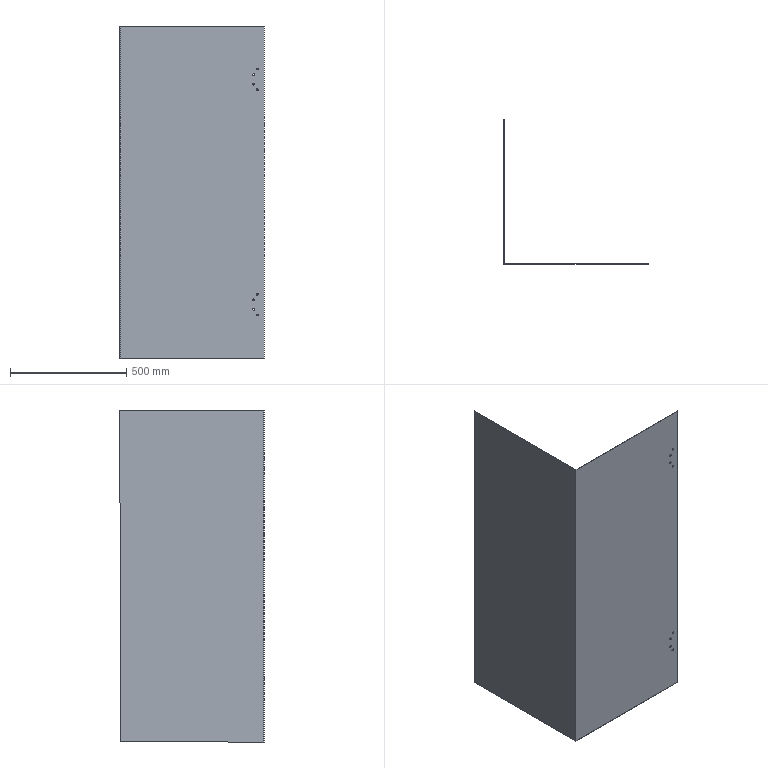Part | SolidWorks | features BaseBody 1 | 1 solid | 24 faces | box 620 x 620 x 1428 mm | volume 3533218 mm3 | cylinder 16 | plane 8 | commonest cylinder face diameters 8.5 x16
STEP:
#1=CARTESIAN_POINT('',(-23.395,-549.023,2695.25));
#2=VERTEX_POINT('',#1);
#3=CARTESIAN_POINT('',(-23.395,-549.023,2686.75));
#4=VERTEX_POINT('',#3);
#5=CARTESIAN_POINT('',(-23.395,-549.023,2691.));
#6=DIRECTION('',(0.,-1.,0.));
#7=DIRECTION('',(0.,0.,-1.));
#8=AXIS2_PLACEMENT_3D('',#5,#6,#7);
#9=CIRCLE('',#8,4.25);
#10=EDGE_CURVE('',#2,#4,#9,.T.);
#11=ORIENTED_EDGE('',*,*,#10,.F.);
#12=CARTESIAN_POINT('',(-23.395,-551.023,2695.25));
#13=VERTEX_POINT('',#12);
#14=CARTESIAN_POINT('',(-23.395,-551.023,2695.25));
#15=DIRECTION('',(0.,-1.,0.));
#16=VECTOR('',#15,1000.);
#17=LINE('',#14,#16);
#18=EDGE_CURVE('',#2,#13,#17,.T.);
#19=ORIENTED_EDGE('',*,*,#18,.T.);
#20=CARTESIAN_POINT('',(-23.395,-551.023,2686.75));
#21=VERTEX_POINT('',#20);
#22=CARTESIAN_POINT('',(-23.395,-551.023,2691.));
#23=DIRECTION('',(0.,-1.,0.));
#24=DIRECTION('',(0.,0.,-1.));
#25=AXIS2_PLACEMENT_3D('',#22,#23,#24);
#26=CIRCLE('',#25,4.25);
#27=EDGE_CURVE('',#13,#21,#26,.T.);
#28=ORIENTED_EDGE('',*,*,#27,.T.);
#29=CARTESIAN_POINT('',(-23.395,-551.023,2686.75));
#30=DIRECTION('',(0.,-1.,0.));
#31=VECTOR('',#30,1000.);
#32=LINE('',#29,#31);
#33=EDGE_CURVE('',#4,#21,#32,.T.);
#34=ORIENTED_EDGE('',*,*,#33,.F.);
#35=EDGE_LOOP('',(#11,#19,#28,#34));
#36=FACE_OUTER_BOUND('',#35,.T.);
#37=CARTESIAN_POINT('',(-23.395,-551.023,2691.));
#38=DIRECTION('',(0.,-1.,0.));
#39=DIRECTION('',(0.,0.,-1.));
#40=AXIS2_PLACEMENT_3D('',#37,#38,#39);
#41=CYLINDRICAL_SURFACE('',#40,4.25);
#42=ADVANCED_FACE('',(#36),#41,.F.);
#43=CARTESIAN_POINT('',(-38.395,-549.023,2670.25));
#44=VERTEX_POINT('',#43);
#45=CARTESIAN_POINT('',(-38.395,-549.023,2661.75));
#46=VERTEX_POINT('',#45);
#47=CARTESIAN_POINT('',(-38.395,-549.023,2666.));
#48=DIRECTION('',(0.,-1.,0.));
#49=DIRECTION('',(0.,0.,-1.));
#50=AXIS2_PLACEMENT_3D('',#47,#48,#49);
#51=CIRCLE('',#50,4.25);
#52=EDGE_CURVE('',#44,#46,#51,.T.);
#53=ORIENTED_EDGE('',*,*,#52,.F.);
#54=CARTESIAN_POINT('',(-38.395,-551.023,2670.25));
#55=VERTEX_POINT('',#54);
#56=CARTESIAN_POINT('',(-38.395,-551.023,2670.25));
#57=DIRECTION('',(0.,-1.,0.));
#58=VECTOR('',#57,1000.);
#59=LINE('',#56,#58);
#60=EDGE_CURVE('',#44,#55,#59,.T.);
#61=ORIENTED_EDGE('',*,*,#60,.T.);
#62=CARTESIAN_POINT('',(-38.395,-551.023,2661.75));
#63=VERTEX_POINT('',#62);
#64=CARTESIAN_POINT('',(-38.395,-551.023,2666.));
#65=DIRECTION('',(0.,-1.,0.));
#66=DIRECTION('',(0.,0.,-1.));
#67=AXIS2_PLACEMENT_3D('',#64,#65,#66);
#68=CIRCLE('',#67,4.25);
#69=EDGE_CURVE('',#55,#63,#68,.T.);
#70=ORIENTED_EDGE('',*,*,#69,.T.);
#71=CARTESIAN_POINT('',(-38.395,-551.023,2661.75));
#72=DIRECTION('',(0.,-1.,0.));
#73=VECTOR('',#72,1000.);
#74=LINE('',#71,#73);
#75=EDGE_CURVE('',#46,#63,#74,.T.);
#76=ORIENTED_EDGE('',*,*,#75,.F.);
#77=EDGE_LOOP('',(#53,#61,#70,#76));
#78=FACE_OUTER_BOUND('',#77,.T.);
#79=CARTESIAN_POINT('',(-38.395,-551.023,2666.));
#80=DIRECTION('',(0.,-1.,0.));
#81=DIRECTION('',(0.,0.,-1.));
#82=AXIS2_PLACEMENT_3D('',#79,#80,#81);
#83=CYLINDRICAL_SURFACE('',#82,4.25);
#84=ADVANCED_FACE('',(#78),#83,.F.);
#85=CARTESIAN_POINT('',(-38.395,-549.023,2630.25));
#86=VERTEX_POINT('',#85);
#87=CARTESIAN_POINT('',(-38.395,-549.023,2621.75));
#88=VERTEX_POINT('',#87);
#89=CARTESIAN_POINT('',(-38.395,-549.023,2626.));
#90=DIRECTION('',(0.,-1.,0.));
#91=DIRECTION('',(0.,0.,-1.));
#92=AXIS2_PLACEMENT_3D('',#89,#90,#91);
#93=CIRCLE('',#92,4.25);
#94=EDGE_CURVE('',#86,#88,#93,.T.);
#95=ORIENTED_EDGE('',*,*,#94,.F.);
#96=CARTESIAN_POINT('',(-38.395,-551.023,2630.25));
#97=VERTEX_POINT('',#96);
#98=CARTESIAN_POINT('',(-38.395,-551.023,2630.25));
#99=DIRECTION('',(0.,-1.,0.));
#100=VECTOR('',#99,1000.);
#101=LINE('',#98,#100);
#102=EDGE_CURVE('',#86,#97,#101,.T.);
#103=ORIENTED_EDGE('',*,*,#102,.T.);
#104=CARTESIAN_POINT('',(-38.395,-551.023,2621.75));
#105=VERTEX_POINT('',#104);
#106=CARTESIAN_POINT('',(-38.395,-551.023,2626.));
#107=DIRECTION('',(0.,-1.,0.));
#108=DIRECTION('',(0.,0.,-1.));
#109=AXIS2_PLACEMENT_3D('',#106,#107,#108);
#110=CIRCLE('',#109,4.25);
#111=EDGE_CURVE('',#97,#105,#110,.T.);
#112=ORIENTED_EDGE('',*,*,#111,.T.);
#113=CARTESIAN_POINT('',(-38.395,-551.023,2621.75));
#114=DIRECTION('',(0.,-1.,0.));
#115=VECTOR('',#114,1000.);
#116=LINE('',#113,#115);
#117=EDGE_CURVE('',#88,#105,#116,.T.);
#118=ORIENTED_EDGE('',*,*,#117,.F.);
#119=EDGE_LOOP('',(#95,#103,#112,#118));
#120=FACE_OUTER_BOUND('',#119,.T.);
#121=CARTESIAN_POINT('',(-38.395,-551.023,2626.));
#122=DIRECTION('',(0.,-1.,0.));
#123=DIRECTION('',(0.,0.,-1.));
#124=AXIS2_PLACEMENT_3D('',#121,#122,#123);
#125=CYLINDRICAL_SURFACE('',#124,4.25);
#126=ADVANCED_FACE('',(#120),#125,.F.);
#127=CARTESIAN_POINT('',(-23.395,-549.023,2605.25));
#128=VERTEX_POINT('',#127);
#129=CARTESIAN_POINT('',(-23.395,-549.023,2596.75));
#130=VERTEX_POINT('',#129);
#131=CARTESIAN_POINT('',(-23.395,-549.023,2601.));
#132=DIRECTION('',(0.,-1.,0.));
#133=DIRECTION('',(0.,0.,-1.));
#134=AXIS2_PLACEMENT_3D('',#131,#132,#133);
#135=CIRCLE('',#134,4.25);
#136=EDGE_CURVE('',#128,#130,#135,.T.);
#137=ORIENTED_EDGE('',*,*,#136,.F.);
#138=CARTESIAN_POINT('',(-23.395,-551.023,2605.25));
#139=VERTEX_POINT('',#138);
#140=CARTESIAN_POINT('',(-23.395,-551.023,2605.25));
#141=DIRECTION('',(0.,-1.,0.));
#142=VECTOR('',#141,1000.);
#143=LINE('',#140,#142);
#144=EDGE_CURVE('',#128,#139,#143,.T.);
#145=ORIENTED_EDGE('',*,*,#144,.T.);
#146=CARTESIAN_POINT('',(-23.395,-551.023,2596.75));
#147=VERTEX_POINT('',#146);
#148=CARTESIAN_POINT('',(-23.395,-551.023,2601.));
#149=DIRECTION('',(0.,-1.,0.));
#150=DIRECTION('',(0.,0.,-1.));
#151=AXIS2_PLACEMENT_3D('',#148,#149,#150);
#152=CIRCLE('',#151,4.25);
#153=EDGE_CURVE('',#139,#147,#152,.T.);
#154=ORIENTED_EDGE('',*,*,#153,.T.);
#155=CARTESIAN_POINT('',(-23.395,-551.023,2596.75));
#156=DIRECTION('',(0.,-1.,0.));
#157=VECTOR('',#156,1000.);
#158=LINE('',#155,#157);
#159=EDGE_CURVE('',#130,#147,#158,.T.);
#160=ORIENTED_EDGE('',*,*,#159,.F.);
#161=EDGE_LOOP('',(#137,#145,#154,#160));
#162=FACE_OUTER_BOUND('',#161,.T.);
#163=CARTESIAN_POINT('',(-23.395,-551.023,2601.));
#164=DIRECTION('',(0.,-1.,0.));
#165=DIRECTION('',(0.,0.,-1.));
#166=AXIS2_PLACEMENT_3D('',#163,#164,#165);
#167=CYLINDRICAL_SURFACE('',#166,4.25);
#168=ADVANCED_FACE('',(#162),#167,.F.);
#169=CARTESIAN_POINT('',(-23.395,-549.023,1727.25));
#170=VERTEX_POINT('',#169);
#171=CARTESIAN_POINT('',(-23.395,-549.023,1718.75));
#172=VERTEX_POINT('',#171);
#173=CARTESIAN_POINT('',(-23.395,-549.023,1723.));
#174=DIRECTION('',(0.,-1.,0.));
#175=DIRECTION('',(0.,0.,-1.));
#176=AXIS2_PLACEMENT_3D('',#173,#174,#175);
#177=CIRCLE('',#176,4.25);
#178=EDGE_CURVE('',#170,#172,#177,.T.);
#179=ORIENTED_EDGE('',*,*,#178,.F.);
#180=CARTESIAN_POINT('',(-23.395,-551.023,1727.25));
#181=VERTEX_POINT('',#180);
#182=CARTESIAN_POINT('',(-23.395,-551.023,1727.25));
#183=DIRECTION('',(0.,-1.,0.));
#184=VECTOR('',#183,1000.);
#185=LINE('',#182,#184);
#186=EDGE_CURVE('',#170,#181,#185,.T.);
#187=ORIENTED_EDGE('',*,*,#186,.T.);
#188=CARTESIAN_POINT('',(-23.395,-551.023,1718.75));
#189=VERTEX_POINT('',#188);
#190=CARTESIAN_POINT('',(-23.395,-551.023,1723.));
#191=DIRECTION('',(0.,-1.,0.));
#192=DIRECTION('',(0.,0.,-1.));
#193=AXIS2_PLACEMENT_3D('',#190,#191,#192);
#194=CIRCLE('',#193,4.25);
#195=EDGE_CURVE('',#181,#189,#194,.T.);
#196=ORIENTED_EDGE('',*,*,#195,.T.);
#197=CARTESIAN_POINT('',(-23.395,-551.023,1718.75));
#198=DIRECTION('',(0.,-1.,0.));
#199=VECTOR('',#198,1000.);
#200=LINE('',#197,#199);
#201=EDGE_CURVE('',#172,#189,#200,.T.);
#202=ORIENTED_EDGE('',*,*,#201,.F.);
#203=EDGE_LOOP('',(#179,#187,#196,#202));
#204=FACE_OUTER_BOUND('',#203,.T.);
#205=CARTESIAN_POINT('',(-23.395,-551.023,1723.));
#206=DIRECTION('',(0.,-1.,0.));
#207=DIRECTION('',(0.,0.,-1.));
#208=AXIS2_PLACEMENT_3D('',#205,#206,#207);
#209=CYLINDRICAL_SURFACE('',#208,4.25);
#210=ADVANCED_FACE('',(#204),#209,.F.);
#211=CARTESIAN_POINT('',(-38.395,-549.023,1702.25));
#212=VERTEX_POINT('',#211);
#213=CARTESIAN_POINT('',(-38.395,-549.023,1693.75));
#214=VERTEX_POINT('',#213);
#215=CARTESIAN_POINT('',(-38.395,-549.023,1698.));
#216=DIRECTION('',(0.,-1.,0.));
#217=DIRECTION('',(0.,0.,-1.));
#218=AXIS2_PLACEMENT_3D('',#215,#216,#217);
#219=CIRCLE('',#218,4.25);
#220=EDGE_CURVE('',#212,#214,#219,.T.);
#221=ORIENTED_EDGE('',*,*,#220,.F.);
#222=CARTESIAN_POINT('',(-38.395,-551.023,1702.25));
#223=VERTEX_POINT('',#222);
#224=CARTESIAN_POINT('',(-38.395,-551.023,1702.25));
#225=DIRECTION('',(0.,-1.,0.));
#226=VECTOR('',#225,1000.);
#227=LINE('',#224,#226);
#228=EDGE_CURVE('',#212,#223,#227,.T.);
#229=ORIENTED_EDGE('',*,*,#228,.T.);
#230=CARTESIAN_POINT('',(-38.395,-551.023,1693.75));
#231=VERTEX_POINT('',#230);
#232=CARTESIAN_POINT('',(-38.395,-551.023,1698.));
#233=DIRECTION('',(0.,-1.,0.));
#234=DIRECTION('',(0.,0.,-1.));
#235=AXIS2_PLACEMENT_3D('',#232,#233,#234);
#236=CIRCLE('',#235,4.25);
#237=EDGE_CURVE('',#223,#231,#236,.T.);
#238=ORIENTED_EDGE('',*,*,#237,.T.);
#239=CARTESIAN_POINT('',(-38.395,-551.023,1693.75));
#240=DIRECTION('',(0.,-1.,0.));
#241=VECTOR('',#240,1000.);
#242=LINE('',#239,#241);
#243=EDGE_CURVE('',#214,#231,#242,.T.);
#244=ORIENTED_EDGE('',*,*,#243,.F.);
#245=EDGE_LOOP('',(#221,#229,#238,#244));
#246=FACE_OUTER_BOUND('',#245,.T.);
#247=CARTESIAN_POINT('',(-38.395,-551.023,1698.));
#248=DIRECTION('',(0.,-1.,0.));
#249=DIRECTION('',(0.,0.,-1.));
#250=AXIS2_PLACEMENT_3D('',#247,#248,#249);
#251=CYLINDRICAL_SURFACE('',#250,4.25);
#252=ADVANCED_FACE('',(#246),#251,.F.);
#253=CARTESIAN_POINT('',(-38.395,-549.023,1662.25));
#254=VERTEX_POINT('',#253);
#255=CARTESIAN_POINT('',(-38.395,-549.023,1653.75));
#256=VERTEX_POINT('',#255);
#257=CARTESIAN_POINT('',(-38.395,-549.023,1658.));
#258=DIRECTION('',(0.,-1.,0.));
#259=DIRECTION('',(0.,0.,-1.));
#260=AXIS2_PLACEMENT_3D('',#257,#258,#259);
#261=CIRCLE('',#260,4.25);
#262=EDGE_CURVE('',#254,#256,#261,.T.);
#263=ORIENTED_EDGE('',*,*,#262,.F.);
#264=CARTESIAN_POINT('',(-38.395,-551.023,1662.25));
#265=VERTEX_POINT('',#264);
#266=CARTESIAN_POINT('',(-38.395,-551.023,1662.25));
#267=DIRECTION('',(0.,-1.,0.));
#268=VECTOR('',#267,1000.);
#269=LINE('',#266,#268);
#270=EDGE_CURVE('',#254,#265,#269,.T.);
#271=ORIENTED_EDGE('',*,*,#270,.T.);
#272=CARTESIAN_POINT('',(-38.395,-551.023,1653.75));
#273=VERTEX_POINT('',#272);
#274=CARTESIAN_POINT('',(-38.395,-551.023,1658.));
#275=DIRECTION('',(0.,-1.,0.));
#276=DIRECTION('',(0.,0.,-1.));
#277=AXIS2_PLACEMENT_3D('',#274,#275,#276);
#278=CIRCLE('',#277,4.25);
#279=EDGE_CURVE('',#265,#273,#278,.T.);
#280=ORIENTED_EDGE('',*,*,#279,.T.);
#281=CARTESIAN_POINT('',(-38.395,-551.023,1653.75));
#282=DIRECTION('',(0.,-1.,0.));
#283=VECTOR('',#282,1000.);
#284=LINE('',#281,#283);
#285=EDGE_CURVE('',#256,#273,#284,.T.);
#286=ORIENTED_EDGE('',*,*,#285,.F.);
#287=EDGE_LOOP('',(#263,#271,#280,#286));
#288=FACE_OUTER_BOUND('',#287,.T.);
#289=CARTESIAN_POINT('',(-38.395,-551.023,1658.));
#290=DIRECTION('',(0.,-1.,0.));
#291=DIRECTION('',(0.,0.,-1.));
#292=AXIS2_PLACEMENT_3D('',#289,#290,#291);
#293=CYLINDRICAL_SURFACE('',#292,4.25);
#294=ADVANCED_FACE('',(#288),#293,.F.);
#295=CARTESIAN_POINT('',(-23.395,-549.023,1637.25));
#296=VERTEX_POINT('',#295);
#297=CARTESIAN_POINT('',(-23.395,-549.023,1628.75));
#298=VERTEX_POINT('',#297);
#299=CARTESIAN_POINT('',(-23.395,-549.023,1633.));
#300=DIRECTION('',(0.,-1.,0.));
#301=DIRECTION('',(0.,0.,-1.));
#302=AXIS2_PLACEMENT_3D('',#299,#300,#301);
#303=CIRCLE('',#302,4.25);
#304=EDGE_CURVE('',#296,#298,#303,.T.);
#305=ORIENTED_EDGE('',*,*,#304,.F.);
#306=CARTESIAN_POINT('',(-23.395,-551.023,1637.25));
#307=VERTEX_POINT('',#306);
#308=CARTESIAN_POINT('',(-23.395,-551.023,1637.25));
#309=DIRECTION('',(0.,-1.,0.));
#310=VECTOR('',#309,1000.);
#311=LINE('',#308,#310);
#312=EDGE_CURVE('',#296,#307,#311,.T.);
#313=ORIENTED_EDGE('',*,*,#312,.T.);
#314=CARTESIAN_POINT('',(-23.395,-551.023,1628.75));
#315=VERTEX_POINT('',#314);
#316=CARTESIAN_POINT('',(-23.395,-551.023,1633.));
#317=DIRECTION('',(0.,-1.,0.));
#318=DIRECTION('',(0.,0.,-1.));
#319=AXIS2_PLACEMENT_3D('',#316,#317,#318);
#320=CIRCLE('',#319,4.25);
#321=EDGE_CURVE('',#307,#315,#320,.T.);
#322=ORIENTED_EDGE('',*,*,#321,.T.);
#323=CARTESIAN_POINT('',(-23.395,-551.023,1628.75));
#324=DIRECTION('',(0.,-1.,0.));
#325=VECTOR('',#324,1000.);
#326=LINE('',#323,#325);
#327=EDGE_CURVE('',#298,#315,#326,.T.);
#328=ORIENTED_EDGE('',*,*,#327,.F.);
#329=EDGE_LOOP('',(#305,#313,#322,#328));
#330=FACE_OUTER_BOUND('',#329,.T.);
#331=CARTESIAN_POINT('',(-23.395,-551.023,1633.));
#332=DIRECTION('',(0.,-1.,0.));
#333=DIRECTION('',(0.,0.,-1.));
#334=AXIS2_PLACEMENT_3D('',#331,#332,#333);
#335=CYLINDRICAL_SURFACE('',#334,4.25);
#336=ADVANCED_FACE('',(#330),#335,.F.);
#337=CARTESIAN_POINT('',(-613.395,67.856,1448.));
#338=VERTEX_POINT('',#337);
#339=CARTESIAN_POINT('',(-611.395,67.856,1448.));
#340=VERTEX_POINT('',#339);
#341=CARTESIAN_POINT('',(-611.395,67.856,1448.));
#342=DIRECTION('',(1.,0.,0.));
#343=VECTOR('',#342,1000.);
#344=LINE('',#341,#343);
#345=EDGE_CURVE('',#338,#340,#344,.T.);
#346=ORIENTED_EDGE('',*,*,#345,.T.);
#347=CARTESIAN_POINT('',(-611.395,-549.023,1448.));
#348=VERTEX_POINT('',#347);
#349=CARTESIAN_POINT('',(-611.395,658.977,1448.));
#350=DIRECTION('',(0.,1.,0.));
#351=VECTOR('',#350,1000.);
#352=LINE('',#349,#351);
#353=EDGE_CURVE('',#348,#340,#352,.T.);
#354=ORIENTED_EDGE('',*,*,#353,.F.);
#355=CARTESIAN_POINT('',(6.605,-549.023,1448.));
#356=VERTEX_POINT('',#355);
#357=CARTESIAN_POINT('',(550.605,-549.023,1448.));
#358=DIRECTION('',(-1.,0.,0.));
#359=VECTOR('',#358,1000.);
#360=LINE('',#357,#359);
#361=EDGE_CURVE('',#356,#348,#360,.T.);
#362=ORIENTED_EDGE('',*,*,#361,.F.);
#363=CARTESIAN_POINT('',(6.605,-551.023,1448.));
#364=VERTEX_POINT('',#363);
#365=CARTESIAN_POINT('',(6.605,556.977,1448.));
#366=DIRECTION('',(0.,1.,0.));
#367=VECTOR('',#366,1000.);
#368=LINE('',#365,#367);
#369=EDGE_CURVE('',#364,#356,#368,.T.);
#370=ORIENTED_EDGE('',*,*,#369,.F.);
#371=CARTESIAN_POINT('',(-613.395,-551.023,1448.));
#372=VERTEX_POINT('',#371);
#373=CARTESIAN_POINT('',(550.605,-551.023,1448.));
#374=DIRECTION('',(-1.,0.,0.));
#375=VECTOR('',#374,1000.);
#376=LINE('',#373,#375);
#377=EDGE_CURVE('',#364,#372,#376,.T.);
#378=ORIENTED_EDGE('',*,*,#377,.T.);
#379=CARTESIAN_POINT('',(-613.395,658.977,1448.));
#380=DIRECTION('',(0.,1.,0.));
#381=VECTOR('',#380,1000.);
#382=LINE('',#379,#381);
#383=EDGE_CURVE('',#372,#338,#382,.T.);
#384=ORIENTED_EDGE('',*,*,#383,.T.);
#385=EDGE_LOOP('',(#346,#354,#362,#370,#378,#384));
#386=FACE_OUTER_BOUND('',#385,.T.);
#387=CARTESIAN_POINT('',(-611.395,556.977,1448.));
#388=DIRECTION('',(0.,0.,1.));
#389=DIRECTION('',(1.,0.,0.));
#390=AXIS2_PLACEMENT_3D('',#387,#388,#389);
#391=PLANE('',#390);
#392=ADVANCED_FACE('',(#386),#391,.F.);
#393=ORIENTED_EDGE('',*,*,#345,.F.);
#394=CARTESIAN_POINT('',(-613.395,68.977,2876.));
#395=VERTEX_POINT('',#394);
#396=CARTESIAN_POINT('',(-613.395,68.978,2876.463));
#397=DIRECTION('',(0.,0.0007854,1.));
#398=VECTOR('',#397,1000.);
#399=LINE('',#396,#398);
#400=EDGE_CURVE('',#338,#395,#399,.T.);
#401=ORIENTED_EDGE('',*,*,#400,.T.);
#402=CARTESIAN_POINT('',(-611.395,68.977,2876.));
#403=VERTEX_POINT('',#402);
#404=CARTESIAN_POINT('',(0.,68.977,2876.));
#405=DIRECTION('',(-1.,0.,0.));
#406=VECTOR('',#405,1000.);
#407=LINE('',#404,#406);
#408=EDGE_CURVE('',#403,#395,#407,.T.);
#409=ORIENTED_EDGE('',*,*,#408,.F.);
#410=CARTESIAN_POINT('',(-611.395,68.978,2876.463));
#411=DIRECTION('',(0.,0.0007854,1.));
#412=VECTOR('',#411,1000.);
#413=LINE('',#410,#412);
#414=EDGE_CURVE('',#340,#403,#413,.T.);
#415=ORIENTED_EDGE('',*,*,#414,.F.);
#416=EDGE_LOOP('',(#393,#401,#409,#415));
#417=FACE_OUTER_BOUND('',#416,.T.);
#418=CARTESIAN_POINT('',(550.615,67.856,1448.));
#419=DIRECTION('',(0.,-1.,0.0007854));
#420=DIRECTION('',(0.,-0.0007854,-1.));
#421=AXIS2_PLACEMENT_3D('',#418,#419,#420);
#422=PLANE('',#421);
#423=ADVANCED_FACE('',(#417),#422,.F.);
#424=CARTESIAN_POINT('',(-611.395,-549.023,2876.));
#425=VERTEX_POINT('',#424);
#426=CARTESIAN_POINT('',(-611.395,-549.023,2876.));
#427=DIRECTION('',(0.,0.,-1.));
#428=VECTOR('',#427,1000.);
#429=LINE('',#426,#428);
#430=EDGE_CURVE('',#425,#348,#429,.T.);
#431=ORIENTED_EDGE('',*,*,#430,.T.);
#432=ORIENTED_EDGE('',*,*,#353,.T.);
#433=ORIENTED_EDGE('',*,*,#414,.T.);
#434=CARTESIAN_POINT('',(-611.395,0.,2876.));
#435=DIRECTION('',(0.,1.,0.));
#436=VECTOR('',#435,1000.);
#437=LINE('',#434,#436);
#438=EDGE_CURVE('',#425,#403,#437,.T.);
#439=ORIENTED_EDGE('',*,*,#438,.F.);
#440=EDGE_LOOP('',(#431,#432,#433,#439));
#441=FACE_OUTER_BOUND('',#440,.T.);
#442=CARTESIAN_POINT('',(-611.395,658.977,2876.));
#443=DIRECTION('',(-1.,0.,0.));
#444=DIRECTION('',(0.,-1.,0.));
#445=AXIS2_PLACEMENT_3D('',#442,#443,#444);
#446=PLANE('',#445);
#447=ADVANCED_FACE('',(#441),#446,.F.);
#448=ORIENTED_EDGE('',*,*,#383,.F.);
#449=CARTESIAN_POINT('',(-613.395,-551.023,2876.));
#450=VERTEX_POINT('',#449);
#451=CARTESIAN_POINT('',(-613.395,-551.023,2876.));
#452=DIRECTION('',(0.,0.,-1.));
#453=VECTOR('',#452,1000.);
#454=LINE('',#451,#453);
#455=EDGE_CURVE('',#450,#372,#454,.T.);
#456=ORIENTED_EDGE('',*,*,#455,.F.);
#457=CARTESIAN_POINT('',(-613.395,658.977,2876.));
#458=DIRECTION('',(0.,1.,0.));
#459=VECTOR('',#458,1000.);
#460=LINE('',#457,#459);
#461=EDGE_CURVE('',#450,#395,#460,.T.);
#462=ORIENTED_EDGE('',*,*,#461,.T.);
#463=ORIENTED_EDGE('',*,*,#400,.F.);
#464=EDGE_LOOP('',(#448,#456,#462,#463));
#465=FACE_OUTER_BOUND('',#464,.T.);
#466=CARTESIAN_POINT('',(-613.395,658.977,2876.));
#467=DIRECTION('',(-1.,0.,0.));
#468=DIRECTION('',(0.,-1.,0.));
#469=AXIS2_PLACEMENT_3D('',#466,#467,#468);
#470=PLANE('',#469);
#471=ADVANCED_FACE('',(#465),#470,.T.);
#472=CARTESIAN_POINT('',(6.605,-549.023,2876.));
#473=VERTEX_POINT('',#472);
#474=CARTESIAN_POINT('',(6.605,-551.023,2876.));
#475=VERTEX_POINT('',#474);
#476=CARTESIAN_POINT('',(6.605,0.,2876.));
#477=DIRECTION('',(0.,-1.,0.));
#478=VECTOR('',#477,1000.);
#479=LINE('',#476,#478);
#480=EDGE_CURVE('',#473,#475,#479,.T.);
#481=ORIENTED_EDGE('',*,*,#480,.F.);
#482=CARTESIAN_POINT('',(0.,-549.023,2876.));
#483=DIRECTION('',(-1.,0.,0.));
#484=VECTOR('',#483,1000.);
#485=LINE('',#482,#484);
#486=EDGE_CURVE('',#473,#425,#485,.T.);
#487=ORIENTED_EDGE('',*,*,#486,.T.);
#488=ORIENTED_EDGE('',*,*,#438,.T.);
#489=ORIENTED_EDGE('',*,*,#408,.T.);
#490=ORIENTED_EDGE('',*,*,#461,.F.);
#491=CARTESIAN_POINT('',(0.,-551.023,2876.));
#492=DIRECTION('',(-1.,0.,0.));
#493=VECTOR('',#492,1000.);
#494=LINE('',#491,#493);
#495=EDGE_CURVE('',#475,#450,#494,.T.);
#496=ORIENTED_EDGE('',*,*,#495,.F.);
#497=EDGE_LOOP('',(#481,#487,#488,#489,#490,#496));
#498=FACE_OUTER_BOUND('',#497,.T.);
#499=CARTESIAN_POINT('',(0.,0.,2876.));
#500=DIRECTION('',(0.,0.,-1.));
#501=DIRECTION('',(-1.,0.,0.));
#502=AXIS2_PLACEMENT_3D('',#499,#500,#501);
#503=PLANE('',#502);
#504=ADVANCED_FACE('',(#498),#503,.F.);
#505=CARTESIAN_POINT('',(-23.395,-551.023,2691.));
#506=DIRECTION('',(0.,-1.,0.));
#507=DIRECTION('',(0.,0.,-1.));
#508=AXIS2_PLACEMENT_3D('',#505,#506,#507);
#509=CIRCLE('',#508,4.25);
#510=EDGE_CURVE('',#21,#13,#509,.T.);
#511=ORIENTED_EDGE('',*,*,#510,.F.);
#512=ORIENTED_EDGE('',*,*,#27,.F.);
#513=EDGE_LOOP('',(#511,#512));
#514=FACE_BOUND('',#513,.T.);
#515=CARTESIAN_POINT('',(-38.395,-551.023,2666.));
#516=DIRECTION('',(0.,-1.,0.));
#517=DIRECTION('',(0.,0.,-1.));
#518=AXIS2_PLACEMENT_3D('',#515,#516,#517);
#519=CIRCLE('',#518,4.25);
#520=EDGE_CURVE('',#63,#55,#519,.T.);
#521=ORIENTED_EDGE('',*,*,#520,.F.);
#522=ORIENTED_EDGE('',*,*,#69,.F.);
#523=EDGE_LOOP('',(#521,#522));
#524=FACE_BOUND('',#523,.T.);
#525=CARTESIAN_POINT('',(-38.395,-551.023,2626.));
#526=DIRECTION('',(0.,-1.,0.));
#527=DIRECTION('',(0.,0.,-1.));
#528=AXIS2_PLACEMENT_3D('',#525,#526,#527);
#529=CIRCLE('',#528,4.25);
#530=EDGE_CURVE('',#105,#97,#529,.T.);
#531=ORIENTED_EDGE('',*,*,#530,.F.);
#532=ORIENTED_EDGE('',*,*,#111,.F.);
#533=EDGE_LOOP('',(#531,#532));
#534=FACE_BOUND('',#533,.T.);
#535=CARTESIAN_POINT('',(-23.395,-551.023,2601.));
#536=DIRECTION('',(0.,-1.,0.));
#537=DIRECTION('',(0.,0.,-1.));
#538=AXIS2_PLACEMENT_3D('',#535,#536,#537);
#539=CIRCLE('',#538,4.25);
#540=EDGE_CURVE('',#147,#139,#539,.T.);
#541=ORIENTED_EDGE('',*,*,#540,.F.);
#542=ORIENTED_EDGE('',*,*,#153,.F.);
#543=EDGE_LOOP('',(#541,#542));
#544=FACE_BOUND('',#543,.T.);
#545=CARTESIAN_POINT('',(-23.395,-551.023,1723.));
#546=DIRECTION('',(0.,-1.,0.));
#547=DIRECTION('',(0.,0.,-1.));
#548=AXIS2_PLACEMENT_3D('',#545,#546,#547);
#549=CIRCLE('',#548,4.25);
#550=EDGE_CURVE('',#189,#181,#549,.T.);
#551=ORIENTED_EDGE('',*,*,#550,.F.);
#552=ORIENTED_EDGE('',*,*,#195,.F.);
#553=EDGE_LOOP('',(#551,#552));
#554=FACE_BOUND('',#553,.T.);
#555=CARTESIAN_POINT('',(-38.395,-551.023,1698.));
#556=DIRECTION('',(0.,-1.,0.));
#557=DIRECTION('',(0.,0.,-1.));
#558=AXIS2_PLACEMENT_3D('',#555,#556,#557);
#559=CIRCLE('',#558,4.25);
#560=EDGE_CURVE('',#231,#223,#559,.T.);
#561=ORIENTED_EDGE('',*,*,#560,.F.);
#562=ORIENTED_EDGE('',*,*,#237,.F.);
#563=EDGE_LOOP('',(#561,#562));
#564=FACE_BOUND('',#563,.T.);
#565=CARTESIAN_POINT('',(-38.395,-551.023,1658.));
#566=DIRECTION('',(0.,-1.,0.));
#567=DIRECTION('',(0.,0.,-1.));
#568=AXIS2_PLACEMENT_3D('',#565,#566,#567);
#569=CIRCLE('',#568,4.25);
#570=EDGE_CURVE('',#273,#265,#569,.T.);
#571=ORIENTED_EDGE('',*,*,#570,.F.);
#572=ORIENTED_EDGE('',*,*,#279,.F.);
#573=EDGE_LOOP('',(#571,#572));
#574=FACE_BOUND('',#573,.T.);
#575=CARTESIAN_POINT('',(-23.395,-551.023,1633.));
#576=DIRECTION('',(0.,-1.,0.));
#577=DIRECTION('',(0.,0.,-1.));
#578=AXIS2_PLACEMENT_3D('',#575,#576,#577);
#579=CIRCLE('',#578,4.25);
#580=EDGE_CURVE('',#315,#307,#579,.T.);
#581=ORIENTED_EDGE('',*,*,#580,.F.);
#582=ORIENTED_EDGE('',*,*,#321,.F.);
#583=EDGE_LOOP('',(#581,#582));
#584=FACE_BOUND('',#583,.T.);
#585=ORIENTED_EDGE('',*,*,#455,.T.);
#586=ORIENTED_EDGE('',*,*,#377,.F.);
#587=CARTESIAN_POINT('',(6.605,-551.023,2876.));
#588=DIRECTION('',(0.,0.,1.));
#589=VECTOR('',#588,1000.);
#590=LINE('',#587,#589);
#591=EDGE_CURVE('',#364,#475,#590,.T.);
#592=ORIENTED_EDGE('',*,*,#591,.T.);
#593=ORIENTED_EDGE('',*,*,#495,.T.);
#594=EDGE_LOOP('',(#585,#586,#592,#593));
#595=FACE_OUTER_BOUND('',#594,.T.);
#596=CARTESIAN_POINT('',(550.605,-551.023,2876.));
#597=DIRECTION('',(0.,-1.,0.));
#598=DIRECTION('',(0.,0.,-1.));
#599=AXIS2_PLACEMENT_3D('',#596,#597,#598);
#600=PLANE('',#599);
#601=ADVANCED_FACE('',(#514,#524,#534,#544,#554,#564,#574,#584,#595),#600,.T.);
#602=CARTESIAN_POINT('',(-23.395,-549.023,2691.));
#603=DIRECTION('',(0.,-1.,0.));
#604=DIRECTION('',(0.,0.,-1.));
#605=AXIS2_PLACEMENT_3D('',#602,#603,#604);
#606=CIRCLE('',#605,4.25);
#607=EDGE_CURVE('',#4,#2,#606,.T.);
#608=ORIENTED_EDGE('',*,*,#607,.T.);
#609=ORIENTED_EDGE('',*,*,#10,.T.);
#610=EDGE_LOOP('',(#608,#609));
#611=FACE_BOUND('',#610,.T.);
#612=CARTESIAN_POINT('',(-38.395,-549.023,2666.));
#613=DIRECTION('',(0.,-1.,0.));
#614=DIRECTION('',(0.,0.,-1.));
#615=AXIS2_PLACEMENT_3D('',#612,#613,#614);
#616=CIRCLE('',#615,4.25);
#617=EDGE_CURVE('',#46,#44,#616,.T.);
#618=ORIENTED_EDGE('',*,*,#617,.T.);
#619=ORIENTED_EDGE('',*,*,#52,.T.);
#620=EDGE_LOOP('',(#618,#619));
#621=FACE_BOUND('',#620,.T.);
#622=CARTESIAN_POINT('',(-38.395,-549.023,2626.));
#623=DIRECTION('',(0.,-1.,0.));
#624=DIRECTION('',(0.,0.,-1.));
#625=AXIS2_PLACEMENT_3D('',#622,#623,#624);
#626=CIRCLE('',#625,4.25);
#627=EDGE_CURVE('',#88,#86,#626,.T.);
#628=ORIENTED_EDGE('',*,*,#627,.T.);
#629=ORIENTED_EDGE('',*,*,#94,.T.);
#630=EDGE_LOOP('',(#628,#629));
#631=FACE_BOUND('',#630,.T.);
#632=CARTESIAN_POINT('',(-23.395,-549.023,2601.));
#633=DIRECTION('',(0.,-1.,0.));
#634=DIRECTION('',(0.,0.,-1.));
#635=AXIS2_PLACEMENT_3D('',#632,#633,#634);
#636=CIRCLE('',#635,4.25);
#637=EDGE_CURVE('',#130,#128,#636,.T.);
#638=ORIENTED_EDGE('',*,*,#637,.T.);
#639=ORIENTED_EDGE('',*,*,#136,.T.);
#640=EDGE_LOOP('',(#638,#639));
#641=FACE_BOUND('',#640,.T.);
#642=CARTESIAN_POINT('',(-23.395,-549.023,1723.));
#643=DIRECTION('',(0.,-1.,0.));
#644=DIRECTION('',(0.,0.,-1.));
#645=AXIS2_PLACEMENT_3D('',#642,#643,#644);
#646=CIRCLE('',#645,4.25);
#647=EDGE_CURVE('',#172,#170,#646,.T.);
#648=ORIENTED_EDGE('',*,*,#647,.T.);
#649=ORIENTED_EDGE('',*,*,#178,.T.);
#650=EDGE_LOOP('',(#648,#649));
#651=FACE_BOUND('',#650,.T.);
#652=CARTESIAN_POINT('',(-38.395,-549.023,1698.));
#653=DIRECTION('',(0.,-1.,0.));
#654=DIRECTION('',(0.,0.,-1.));
#655=AXIS2_PLACEMENT_3D('',#652,#653,#654);
#656=CIRCLE('',#655,4.25);
#657=EDGE_CURVE('',#214,#212,#656,.T.);
#658=ORIENTED_EDGE('',*,*,#657,.T.);
#659=ORIENTED_EDGE('',*,*,#220,.T.);
#660=EDGE_LOOP('',(#658,#659));
#661=FACE_BOUND('',#660,.T.);
#662=CARTESIAN_POINT('',(-38.395,-549.023,1658.));
#663=DIRECTION('',(0.,-1.,0.));
#664=DIRECTION('',(0.,0.,-1.));
#665=AXIS2_PLACEMENT_3D('',#662,#663,#664);
#666=CIRCLE('',#665,4.25);
#667=EDGE_CURVE('',#256,#254,#666,.T.);
#668=ORIENTED_EDGE('',*,*,#667,.T.);
#669=ORIENTED_EDGE('',*,*,#262,.T.);
#670=EDGE_LOOP('',(#668,#669));
#671=FACE_BOUND('',#670,.T.);
#672=CARTESIAN_POINT('',(-23.395,-549.023,1633.));
#673=DIRECTION('',(0.,-1.,0.));
#674=DIRECTION('',(0.,0.,-1.));
#675=AXIS2_PLACEMENT_3D('',#672,#673,#674);
#676=CIRCLE('',#675,4.25);
#677=EDGE_CURVE('',#298,#296,#676,.T.);
#678=ORIENTED_EDGE('',*,*,#677,.T.);
#679=ORIENTED_EDGE('',*,*,#304,.T.);
#680=EDGE_LOOP('',(#678,#679));
#681=FACE_BOUND('',#680,.T.);
#682=CARTESIAN_POINT('',(6.605,-549.023,2876.));
#683=DIRECTION('',(0.,0.,1.));
#684=VECTOR('',#683,1000.);
#685=LINE('',#682,#684);
#686=EDGE_CURVE('',#356,#473,#685,.T.);
#687=ORIENTED_EDGE('',*,*,#686,.F.);
#688=ORIENTED_EDGE('',*,*,#361,.T.);
#689=ORIENTED_EDGE('',*,*,#430,.F.);
#690=ORIENTED_EDGE('',*,*,#486,.F.);
#691=EDGE_LOOP('',(#687,#688,#689,#690));
#692=FACE_OUTER_BOUND('',#691,.T.);
#693=CARTESIAN_POINT('',(550.605,-549.023,2876.));
#694=DIRECTION('',(0.,-1.,0.));
#695=DIRECTION('',(0.,0.,-1.));
#696=AXIS2_PLACEMENT_3D('',#693,#694,#695);
#697=PLANE('',#696);
#698=ADVANCED_FACE('',(#611,#621,#631,#641,#651,#661,#671,#681,#692),#697,.F.);
#699=ORIENTED_EDGE('',*,*,#369,.T.);
#700=ORIENTED_EDGE('',*,*,#686,.T.);
#701=ORIENTED_EDGE('',*,*,#480,.T.);
#702=ORIENTED_EDGE('',*,*,#591,.F.);
#703=EDGE_LOOP('',(#699,#700,#701,#702));
#704=FACE_OUTER_BOUND('',#703,.T.);
#705=CARTESIAN_POINT('',(6.605,-551.033,2950.727));
#706=DIRECTION('',(1.,0.,0.));
#707=DIRECTION('',(0.,0.,-1.));
#708=AXIS2_PLACEMENT_3D('',#705,#706,#707);
#709=PLANE('',#708);
#710=ADVANCED_FACE('',(#704),#709,.T.);
#711=ORIENTED_EDGE('',*,*,#312,.F.);
#712=ORIENTED_EDGE('',*,*,#677,.F.);
#713=ORIENTED_EDGE('',*,*,#327,.T.);
#714=ORIENTED_EDGE('',*,*,#580,.T.);
#715=EDGE_LOOP('',(#711,#712,#713,#714));
#716=FACE_OUTER_BOUND('',#715,.T.);
#717=CARTESIAN_POINT('',(-23.395,-551.023,1633.));
#718=DIRECTION('',(0.,-1.,0.));
#719=DIRECTION('',(0.,0.,-1.));
#720=AXIS2_PLACEMENT_3D('',#717,#718,#719);
#721=CYLINDRICAL_SURFACE('',#720,4.25);
#722=ADVANCED_FACE('',(#716),#721,.F.);
#723=ORIENTED_EDGE('',*,*,#270,.F.);
#724=ORIENTED_EDGE('',*,*,#667,.F.);
#725=ORIENTED_EDGE('',*,*,#285,.T.);
#726=ORIENTED_EDGE('',*,*,#570,.T.);
#727=EDGE_LOOP('',(#723,#724,#725,#726));
#728=FACE_OUTER_BOUND('',#727,.T.);
#729=CARTESIAN_POINT('',(-38.395,-551.023,1658.));
#730=DIRECTION('',(0.,-1.,0.));
#731=DIRECTION('',(0.,0.,-1.));
#732=AXIS2_PLACEMENT_3D('',#729,#730,#731);
#733=CYLINDRICAL_SURFACE('',#732,4.25);
#734=ADVANCED_FACE('',(#728),#733,.F.);
#735=ORIENTED_EDGE('',*,*,#228,.F.);
#736=ORIENTED_EDGE('',*,*,#657,.F.);
#737=ORIENTED_EDGE('',*,*,#243,.T.);
#738=ORIENTED_EDGE('',*,*,#560,.T.);
#739=EDGE_LOOP('',(#735,#736,#737,#738));
#740=FACE_OUTER_BOUND('',#739,.T.);
#741=CARTESIAN_POINT('',(-38.395,-551.023,1698.));
#742=DIRECTION('',(0.,-1.,0.));
#743=DIRECTION('',(0.,0.,-1.));
#744=AXIS2_PLACEMENT_3D('',#741,#742,#743);
#745=CYLINDRICAL_SURFACE('',#744,4.25);
#746=ADVANCED_FACE('',(#740),#745,.F.);
#747=ORIENTED_EDGE('',*,*,#186,.F.);
#748=ORIENTED_EDGE('',*,*,#647,.F.);
#749=ORIENTED_EDGE('',*,*,#201,.T.);
#750=ORIENTED_EDGE('',*,*,#550,.T.);
#751=EDGE_LOOP('',(#747,#748,#749,#750));
#752=FACE_OUTER_BOUND('',#751,.T.);
#753=CARTESIAN_POINT('',(-23.395,-551.023,1723.));
#754=DIRECTION('',(0.,-1.,0.));
#755=DIRECTION('',(0.,0.,-1.));
#756=AXIS2_PLACEMENT_3D('',#753,#754,#755);
#757=CYLINDRICAL_SURFACE('',#756,4.25);
#758=ADVANCED_FACE('',(#752),#757,.F.);
#759=ORIENTED_EDGE('',*,*,#144,.F.);
#760=ORIENTED_EDGE('',*,*,#637,.F.);
#761=ORIENTED_EDGE('',*,*,#159,.T.);
#762=ORIENTED_EDGE('',*,*,#540,.T.);
#763=EDGE_LOOP('',(#759,#760,#761,#762));
#764=FACE_OUTER_BOUND('',#763,.T.);
#765=CARTESIAN_POINT('',(-23.395,-551.023,2601.));
#766=DIRECTION('',(0.,-1.,0.));
#767=DIRECTION('',(0.,0.,-1.));
#768=AXIS2_PLACEMENT_3D('',#765,#766,#767);
#769=CYLINDRICAL_SURFACE('',#768,4.25);
#770=ADVANCED_FACE('',(#764),#769,.F.);
#771=ORIENTED_EDGE('',*,*,#102,.F.);
#772=ORIENTED_EDGE('',*,*,#627,.F.);
#773=ORIENTED_EDGE('',*,*,#117,.T.);
#774=ORIENTED_EDGE('',*,*,#530,.T.);
#775=EDGE_LOOP('',(#771,#772,#773,#774));
#776=FACE_OUTER_BOUND('',#775,.T.);
#777=CARTESIAN_POINT('',(-38.395,-551.023,2626.));
#778=DIRECTION('',(0.,-1.,0.));
#779=DIRECTION('',(0.,0.,-1.));
#780=AXIS2_PLACEMENT_3D('',#777,#778,#779);
#781=CYLINDRICAL_SURFACE('',#780,4.25);
#782=ADVANCED_FACE('',(#776),#781,.F.);
#783=ORIENTED_EDGE('',*,*,#60,.F.);
#784=ORIENTED_EDGE('',*,*,#617,.F.);
#785=ORIENTED_EDGE('',*,*,#75,.T.);
#786=ORIENTED_EDGE('',*,*,#520,.T.);
#787=EDGE_LOOP('',(#783,#784,#785,#786));
#788=FACE_OUTER_BOUND('',#787,.T.);
#789=CARTESIAN_POINT('',(-38.395,-551.023,2666.));
#790=DIRECTION('',(0.,-1.,0.));
#791=DIRECTION('',(0.,0.,-1.));
#792=AXIS2_PLACEMENT_3D('',#789,#790,#791);
#793=CYLINDRICAL_SURFACE('',#792,4.25);
#794=ADVANCED_FACE('',(#788),#793,.F.);
#795=ORIENTED_EDGE('',*,*,#18,.F.);
#796=ORIENTED_EDGE('',*,*,#607,.F.);
#797=ORIENTED_EDGE('',*,*,#33,.T.);
#798=ORIENTED_EDGE('',*,*,#510,.T.);
#799=EDGE_LOOP('',(#795,#796,#797,#798));
#800=FACE_OUTER_BOUND('',#799,.T.);
#801=CARTESIAN_POINT('',(-23.395,-551.023,2691.));
#802=DIRECTION('',(0.,-1.,0.));
#803=DIRECTION('',(0.,0.,-1.));
#804=AXIS2_PLACEMENT_3D('',#801,#802,#803);
#805=CYLINDRICAL_SURFACE('',#804,4.25);
#806=ADVANCED_FACE('',(#800),#805,.F.);
#807=CLOSED_SHELL('',(#42,#84,#126,#168,#210,#252,#294,#336,#392,#423,#447,#471,#504,#601,#698,#710,#722,#734,#746,#758,#770,#782,#794,#806));
#808=MANIFOLD_SOLID_BREP('',#807);
#809=CARTESIAN_POINT('',(0.,0.,0.));
#810=DIRECTION('',(0.,0.,1.));
#811=DIRECTION('',(1.,0.,0.));
#812=AXIS2_PLACEMENT_3D('',#809,#810,#811);
#813=(LENGTH_UNIT()NAMED_UNIT(*)SI_UNIT(.MILLI.,.METRE.));
#814=UNCERTAINTY_MEASURE_WITH_UNIT(LENGTH_MEASURE(0.00001),#813,'','');
#815=(NAMED_UNIT(*)PLANE_ANGLE_UNIT()SI_UNIT($,.RADIAN.));
#816=(NAMED_UNIT(*)SI_UNIT($,.STERADIAN.)SOLID_ANGLE_UNIT());
#817=(GEOMETRIC_REPRESENTATION_CONTEXT(3)GLOBAL_UNCERTAINTY_ASSIGNED_CONTEXT((#814))GLOBAL_UNIT_ASSIGNED_CONTEXT((#813,#815,#816))REPRESENTATION_CONTEXT('',''));
#818=ADVANCED_BREP_SHAPE_REPRESENTATION('',(#808,#812),#817);